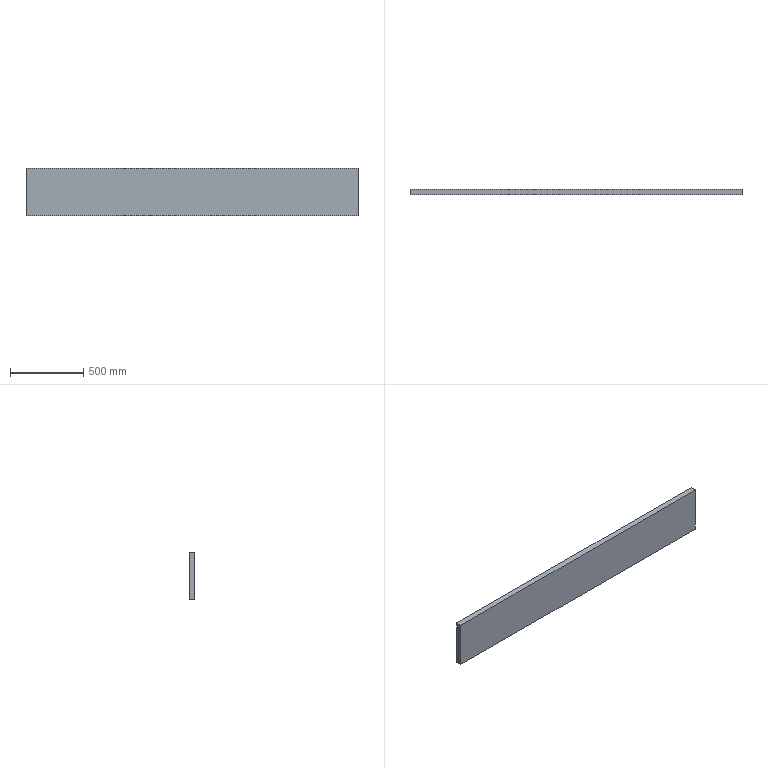Part | SolidWorks | features Extrusion 1 | 1 solid | 6 faces | box 2266 x 40 x 327.5 mm | volume 29684600 mm3 | plane 6
STEP:
#1=CARTESIAN_POINT('',(1133.,0.,163.75));
#2=VERTEX_POINT('',#1);
#3=CARTESIAN_POINT('',(1133.,0.,-163.75));
#4=VERTEX_POINT('',#3);
#5=CARTESIAN_POINT('',(1133.,0.,163.75));
#6=DIRECTION('',(0.,0.,-1.));
#7=VECTOR('',#6,1000.);
#8=LINE('',#5,#7);
#9=EDGE_CURVE('',#2,#4,#8,.T.);
#10=ORIENTED_EDGE('',*,*,#9,.T.);
#11=CARTESIAN_POINT('',(1133.,40.,-163.75));
#12=VERTEX_POINT('',#11);
#13=CARTESIAN_POINT('',(1133.,40.,-163.75));
#14=DIRECTION('',(0.,-1.,0.));
#15=VECTOR('',#14,1000.);
#16=LINE('',#13,#15);
#17=EDGE_CURVE('',#12,#4,#16,.T.);
#18=ORIENTED_EDGE('',*,*,#17,.F.);
#19=CARTESIAN_POINT('',(1133.,40.,163.75));
#20=VERTEX_POINT('',#19);
#21=CARTESIAN_POINT('',(1133.,40.,163.75));
#22=DIRECTION('',(0.,0.,-1.));
#23=VECTOR('',#22,1000.);
#24=LINE('',#21,#23);
#25=EDGE_CURVE('',#20,#12,#24,.T.);
#26=ORIENTED_EDGE('',*,*,#25,.F.);
#27=CARTESIAN_POINT('',(1133.,40.,163.75));
#28=DIRECTION('',(0.,-1.,0.));
#29=VECTOR('',#28,1000.);
#30=LINE('',#27,#29);
#31=EDGE_CURVE('',#20,#2,#30,.T.);
#32=ORIENTED_EDGE('',*,*,#31,.T.);
#33=EDGE_LOOP('',(#10,#18,#26,#32));
#34=FACE_OUTER_BOUND('',#33,.T.);
#35=CARTESIAN_POINT('',(1133.,40.,163.75));
#36=DIRECTION('',(-1.,0.,0.));
#37=DIRECTION('',(0.,0.,1.));
#38=AXIS2_PLACEMENT_3D('',#35,#36,#37);
#39=PLANE('',#38);
#40=ADVANCED_FACE('',(#34),#39,.F.);
#41=CARTESIAN_POINT('',(-1133.,0.,-163.75));
#42=VERTEX_POINT('',#41);
#43=CARTESIAN_POINT('',(-1133.,0.,-163.75));
#44=DIRECTION('',(-1.,0.,0.));
#45=VECTOR('',#44,1000.);
#46=LINE('',#43,#45);
#47=EDGE_CURVE('',#4,#42,#46,.T.);
#48=ORIENTED_EDGE('',*,*,#47,.T.);
#49=CARTESIAN_POINT('',(-1133.,40.,-163.75));
#50=VERTEX_POINT('',#49);
#51=CARTESIAN_POINT('',(-1133.,40.,-163.75));
#52=DIRECTION('',(0.,-1.,0.));
#53=VECTOR('',#52,1000.);
#54=LINE('',#51,#53);
#55=EDGE_CURVE('',#50,#42,#54,.T.);
#56=ORIENTED_EDGE('',*,*,#55,.F.);
#57=CARTESIAN_POINT('',(-1133.,40.,-163.75));
#58=DIRECTION('',(-1.,0.,0.));
#59=VECTOR('',#58,1000.);
#60=LINE('',#57,#59);
#61=EDGE_CURVE('',#12,#50,#60,.T.);
#62=ORIENTED_EDGE('',*,*,#61,.F.);
#63=ORIENTED_EDGE('',*,*,#17,.T.);
#64=EDGE_LOOP('',(#48,#56,#62,#63));
#65=FACE_OUTER_BOUND('',#64,.T.);
#66=CARTESIAN_POINT('',(-1133.,40.,-163.75));
#67=DIRECTION('',(0.,0.,1.));
#68=DIRECTION('',(1.,0.,0.));
#69=AXIS2_PLACEMENT_3D('',#66,#67,#68);
#70=PLANE('',#69);
#71=ADVANCED_FACE('',(#65),#70,.F.);
#72=CARTESIAN_POINT('',(-1133.,0.,163.75));
#73=VERTEX_POINT('',#72);
#74=CARTESIAN_POINT('',(-1133.,0.,163.75));
#75=DIRECTION('',(0.,0.,1.));
#76=VECTOR('',#75,1000.);
#77=LINE('',#74,#76);
#78=EDGE_CURVE('',#42,#73,#77,.T.);
#79=ORIENTED_EDGE('',*,*,#78,.T.);
#80=CARTESIAN_POINT('',(-1133.,40.,163.75));
#81=VERTEX_POINT('',#80);
#82=CARTESIAN_POINT('',(-1133.,40.,163.75));
#83=DIRECTION('',(0.,-1.,0.));
#84=VECTOR('',#83,1000.);
#85=LINE('',#82,#84);
#86=EDGE_CURVE('',#81,#73,#85,.T.);
#87=ORIENTED_EDGE('',*,*,#86,.F.);
#88=CARTESIAN_POINT('',(-1133.,40.,163.75));
#89=DIRECTION('',(0.,0.,1.));
#90=VECTOR('',#89,1000.);
#91=LINE('',#88,#90);
#92=EDGE_CURVE('',#50,#81,#91,.T.);
#93=ORIENTED_EDGE('',*,*,#92,.F.);
#94=ORIENTED_EDGE('',*,*,#55,.T.);
#95=EDGE_LOOP('',(#79,#87,#93,#94));
#96=FACE_OUTER_BOUND('',#95,.T.);
#97=CARTESIAN_POINT('',(-1133.,40.,163.75));
#98=DIRECTION('',(1.,0.,0.));
#99=DIRECTION('',(0.,0.,-1.));
#100=AXIS2_PLACEMENT_3D('',#97,#98,#99);
#101=PLANE('',#100);
#102=ADVANCED_FACE('',(#96),#101,.F.);
#103=CARTESIAN_POINT('',(-1133.,0.,163.75));
#104=DIRECTION('',(1.,0.,0.));
#105=VECTOR('',#104,1000.);
#106=LINE('',#103,#105);
#107=EDGE_CURVE('',#73,#2,#106,.T.);
#108=ORIENTED_EDGE('',*,*,#107,.T.);
#109=ORIENTED_EDGE('',*,*,#31,.F.);
#110=CARTESIAN_POINT('',(-1133.,40.,163.75));
#111=DIRECTION('',(1.,0.,0.));
#112=VECTOR('',#111,1000.);
#113=LINE('',#110,#112);
#114=EDGE_CURVE('',#81,#20,#113,.T.);
#115=ORIENTED_EDGE('',*,*,#114,.F.);
#116=ORIENTED_EDGE('',*,*,#86,.T.);
#117=EDGE_LOOP('',(#108,#109,#115,#116));
#118=FACE_OUTER_BOUND('',#117,.T.);
#119=CARTESIAN_POINT('',(-1133.,40.,163.75));
#120=DIRECTION('',(0.,0.,-1.));
#121=DIRECTION('',(-1.,0.,0.));
#122=AXIS2_PLACEMENT_3D('',#119,#120,#121);
#123=PLANE('',#122);
#124=ADVANCED_FACE('',(#118),#123,.F.);
#125=ORIENTED_EDGE('',*,*,#25,.T.);
#126=ORIENTED_EDGE('',*,*,#61,.T.);
#127=ORIENTED_EDGE('',*,*,#92,.T.);
#128=ORIENTED_EDGE('',*,*,#114,.T.);
#129=EDGE_LOOP('',(#125,#126,#127,#128));
#130=FACE_OUTER_BOUND('',#129,.T.);
#131=CARTESIAN_POINT('',(0.,40.,0.));
#132=DIRECTION('',(0.,-1.,0.));
#133=DIRECTION('',(0.,0.,-1.));
#134=AXIS2_PLACEMENT_3D('',#131,#132,#133);
#135=PLANE('',#134);
#136=ADVANCED_FACE('',(#130),#135,.F.);
#137=ORIENTED_EDGE('',*,*,#9,.F.);
#138=ORIENTED_EDGE('',*,*,#107,.F.);
#139=ORIENTED_EDGE('',*,*,#78,.F.);
#140=ORIENTED_EDGE('',*,*,#47,.F.);
#141=EDGE_LOOP('',(#137,#138,#139,#140));
#142=FACE_OUTER_BOUND('',#141,.T.);
#143=CARTESIAN_POINT('',(0.,0.,0.));
#144=DIRECTION('',(0.,-1.,0.));
#145=DIRECTION('',(0.,0.,-1.));
#146=AXIS2_PLACEMENT_3D('',#143,#144,#145);
#147=PLANE('',#146);
#148=ADVANCED_FACE('',(#142),#147,.T.);
#149=CLOSED_SHELL('',(#40,#71,#102,#124,#136,#148));
#150=MANIFOLD_SOLID_BREP('',#149);
#151=CARTESIAN_POINT('',(0.,0.,0.));
#152=DIRECTION('',(0.,0.,1.));
#153=DIRECTION('',(1.,0.,0.));
#154=AXIS2_PLACEMENT_3D('',#151,#152,#153);
#155=(LENGTH_UNIT()NAMED_UNIT(*)SI_UNIT(.MILLI.,.METRE.));
#156=UNCERTAINTY_MEASURE_WITH_UNIT(LENGTH_MEASURE(0.00001),#155,'','');
#157=(NAMED_UNIT(*)PLANE_ANGLE_UNIT()SI_UNIT($,.RADIAN.));
#158=(NAMED_UNIT(*)SI_UNIT($,.STERADIAN.)SOLID_ANGLE_UNIT());
#159=(GEOMETRIC_REPRESENTATION_CONTEXT(3)GLOBAL_UNCERTAINTY_ASSIGNED_CONTEXT((#156))GLOBAL_UNIT_ASSIGNED_CONTEXT((#155,#157,#158))REPRESENTATION_CONTEXT('',''));
#160=ADVANCED_BREP_SHAPE_REPRESENTATION('',(#150,#154),#159);